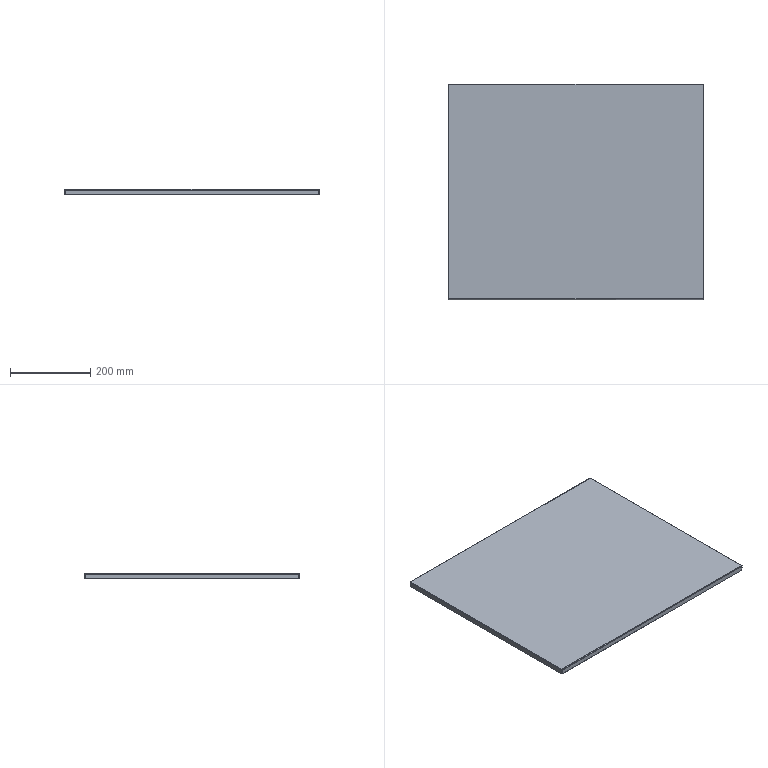Part | STEP file | Part 3^Frame unit | 1 solid | 38 faces | box 638 x 538 x 13.5 mm | volume 554979 mm3 | plane 22 | spline 8 | cylinder 8 | commonest cylinder face diameters 1 x4 4 x4
STEP:
#1=CARTESIAN_POINT('',(-317.,83.,-1.5));
#2=VERTEX_POINT('',#1);
#3=CARTESIAN_POINT('',(317.,83.,-1.5));
#4=VERTEX_POINT('',#3);
#5=CARTESIAN_POINT('',(-317.,83.,-1.5));
#6=DIRECTION('',(1.,0.,0.));
#7=VECTOR('',#6,1000.);
#8=LINE('',#5,#7);
#9=EDGE_CURVE('',#2,#4,#8,.T.);
#10=ORIENTED_EDGE('',*,*,#9,.F.);
#11=CARTESIAN_POINT('',(-317.,617.,-1.5));
#12=VERTEX_POINT('',#11);
#13=CARTESIAN_POINT('',(-317.,617.,-1.5));
#14=DIRECTION('',(0.,-1.,0.));
#15=VECTOR('',#14,1000.);
#16=LINE('',#13,#15);
#17=EDGE_CURVE('',#12,#2,#16,.T.);
#18=ORIENTED_EDGE('',*,*,#17,.F.);
#19=CARTESIAN_POINT('',(317.,617.,-1.5));
#20=VERTEX_POINT('',#19);
#21=CARTESIAN_POINT('',(317.,617.,-1.5));
#22=DIRECTION('',(-1.,0.,0.));
#23=VECTOR('',#22,1000.);
#24=LINE('',#21,#23);
#25=EDGE_CURVE('',#20,#12,#24,.T.);
#26=ORIENTED_EDGE('',*,*,#25,.F.);
#27=CARTESIAN_POINT('',(317.,83.,-1.5));
#28=DIRECTION('',(0.,1.,0.));
#29=VECTOR('',#28,1000.);
#30=LINE('',#27,#29);
#31=EDGE_CURVE('',#4,#20,#30,.T.);
#32=ORIENTED_EDGE('',*,*,#31,.F.);
#33=EDGE_LOOP('',(#10,#18,#26,#32));
#34=FACE_OUTER_BOUND('',#33,.T.);
#35=CARTESIAN_POINT('',(0.,0.,-1.5));
#36=DIRECTION('',(0.,0.,1.));
#37=DIRECTION('',(1.,0.,0.));
#38=AXIS2_PLACEMENT_3D('',#35,#36,#37);
#39=PLANE('',#38);
#40=ADVANCED_FACE('',(#34),#39,.F.);
#41=CARTESIAN_POINT('',(-317.,617.,0.));
#42=VERTEX_POINT('',#41);
#43=CARTESIAN_POINT('',(-317.,83.,0.));
#44=VERTEX_POINT('',#43);
#45=CARTESIAN_POINT('',(-317.,617.,0.));
#46=DIRECTION('',(0.,-1.,0.));
#47=VECTOR('',#46,1000.);
#48=LINE('',#45,#47);
#49=EDGE_CURVE('',#42,#44,#48,.T.);
#50=ORIENTED_EDGE('',*,*,#49,.T.);
#51=CARTESIAN_POINT('',(317.,83.,0.));
#52=VERTEX_POINT('',#51);
#53=CARTESIAN_POINT('',(-317.,83.,0.));
#54=DIRECTION('',(1.,0.,0.));
#55=VECTOR('',#54,1000.);
#56=LINE('',#53,#55);
#57=EDGE_CURVE('',#44,#52,#56,.T.);
#58=ORIENTED_EDGE('',*,*,#57,.T.);
#59=CARTESIAN_POINT('',(317.,617.,0.));
#60=VERTEX_POINT('',#59);
#61=CARTESIAN_POINT('',(317.,83.,0.));
#62=DIRECTION('',(0.,1.,0.));
#63=VECTOR('',#62,1000.);
#64=LINE('',#61,#63);
#65=EDGE_CURVE('',#52,#60,#64,.T.);
#66=ORIENTED_EDGE('',*,*,#65,.T.);
#67=CARTESIAN_POINT('',(317.,617.,0.));
#68=DIRECTION('',(-1.,0.,0.));
#69=VECTOR('',#68,1000.);
#70=LINE('',#67,#69);
#71=EDGE_CURVE('',#60,#42,#70,.T.);
#72=ORIENTED_EDGE('',*,*,#71,.T.);
#73=EDGE_LOOP('',(#50,#58,#66,#72));
#74=FACE_OUTER_BOUND('',#73,.T.);
#75=CARTESIAN_POINT('',(0.,0.,0.));
#76=DIRECTION('',(0.,0.,1.));
#77=DIRECTION('',(1.,0.,0.));
#78=AXIS2_PLACEMENT_3D('',#75,#76,#77);
#79=PLANE('',#78);
#80=ADVANCED_FACE('',(#74),#79,.T.);
#81=CARTESIAN_POINT('',(-316.793,619.,-2.));
#82=VERTEX_POINT('',#81);
#83=CARTESIAN_POINT('',(-316.793,617.5,-2.));
#84=VERTEX_POINT('',#83);
#85=CARTESIAN_POINT('',(-316.793,617.5,-2.));
#86=DIRECTION('',(0.,-1.,0.));
#87=VECTOR('',#86,1000.);
#88=LINE('',#85,#87);
#89=EDGE_CURVE('',#82,#84,#88,.T.);
#90=ORIENTED_EDGE('',*,*,#89,.T.);
#91=CARTESIAN_POINT('',(-317.,617.,-1.5));
#92=CARTESIAN_POINT('',(-316.965,617.131,-1.5));
#93=CARTESIAN_POINT('',(-316.931,617.261,-1.554));
#94=CARTESIAN_POINT('',(-316.862,617.446,-1.739));
#95=CARTESIAN_POINT('',(-316.827,617.5,-1.869));
#96=CARTESIAN_POINT('',(-316.793,617.5,-2.));
#97=B_SPLINE_CURVE_WITH_KNOTS('',3,(#91,#92,#93,#94,#95,#96),.UNSPECIFIED.,.F.,.F.,(4,2,4),(0.,0.5,1.),.UNSPECIFIED.);
#98=EDGE_CURVE('',#12,#84,#97,.T.);
#99=ORIENTED_EDGE('',*,*,#98,.F.);
#100=CARTESIAN_POINT('',(-317.,617.,-1.5));
#101=DIRECTION('',(0.,0.,1.));
#102=VECTOR('',#101,1000.);
#103=LINE('',#100,#102);
#104=EDGE_CURVE('',#12,#42,#103,.T.);
#105=ORIENTED_EDGE('',*,*,#104,.T.);
#106=CARTESIAN_POINT('',(-317.,617.,0.));
#107=CARTESIAN_POINT('',(-316.983,617.262,0.));
#108=CARTESIAN_POINT('',(-316.965,617.523,-0.05205));
#109=CARTESIAN_POINT('',(-316.931,618.007,-0.2524));
#110=CARTESIAN_POINT('',(-316.914,618.229,-0.4007));
#111=CARTESIAN_POINT('',(-316.879,618.599,-0.7709));
#112=CARTESIAN_POINT('',(-316.862,618.748,-0.9928));
#113=CARTESIAN_POINT('',(-316.827,618.948,-1.477));
#114=CARTESIAN_POINT('',(-316.81,619.,-1.738));
#115=CARTESIAN_POINT('',(-316.793,619.,-2.));
#116=B_SPLINE_CURVE_WITH_KNOTS('',3,(#106,#107,#108,#109,#110,#111,#112,#113,#114,#115),.UNSPECIFIED.,.F.,.F.,(4,2,2,2,4),(0.,0.25,0.5,0.75,1.),.UNSPECIFIED.);
#117=EDGE_CURVE('',#42,#82,#116,.T.);
#118=ORIENTED_EDGE('',*,*,#117,.T.);
#119=EDGE_LOOP('',(#90,#99,#105,#118));
#120=FACE_OUTER_BOUND('',#119,.T.);
#121=CARTESIAN_POINT('',(-317.,617.,0.015));
#122=CARTESIAN_POINT('',(-316.983,617.264,0.015));
#123=CARTESIAN_POINT('',(-316.965,617.527,-0.03745));
#124=CARTESIAN_POINT('',(-316.931,618.015,-0.2393));
#125=CARTESIAN_POINT('',(-316.914,618.238,-0.3887));
#126=CARTESIAN_POINT('',(-316.879,618.611,-0.7617));
#127=CARTESIAN_POINT('',(-316.862,618.761,-0.9852));
#128=CARTESIAN_POINT('',(-316.827,618.963,-1.473));
#129=CARTESIAN_POINT('',(-316.81,619.015,-1.736));
#130=CARTESIAN_POINT('',(-316.793,619.015,-2.));
#131=CARTESIAN_POINT('',(-317.,617.,0.));
#132=CARTESIAN_POINT('',(-316.983,617.262,0.));
#133=CARTESIAN_POINT('',(-316.965,617.523,-0.05205));
#134=CARTESIAN_POINT('',(-316.931,618.007,-0.2524));
#135=CARTESIAN_POINT('',(-316.914,618.229,-0.4007));
#136=CARTESIAN_POINT('',(-316.879,618.599,-0.7709));
#137=CARTESIAN_POINT('',(-316.862,618.748,-0.9928));
#138=CARTESIAN_POINT('',(-316.827,618.948,-1.477));
#139=CARTESIAN_POINT('',(-316.81,619.,-1.738));
#140=CARTESIAN_POINT('',(-316.793,619.,-2.));
#141=CARTESIAN_POINT('',(-317.,617.,-1.5));
#142=CARTESIAN_POINT('',(-316.983,617.065,-1.5));
#143=CARTESIAN_POINT('',(-316.965,617.131,-1.513));
#144=CARTESIAN_POINT('',(-316.931,617.252,-1.563));
#145=CARTESIAN_POINT('',(-316.914,617.307,-1.6));
#146=CARTESIAN_POINT('',(-316.879,617.4,-1.693));
#147=CARTESIAN_POINT('',(-316.862,617.437,-1.748));
#148=CARTESIAN_POINT('',(-316.827,617.487,-1.869));
#149=CARTESIAN_POINT('',(-316.81,617.5,-1.935));
#150=CARTESIAN_POINT('',(-316.793,617.5,-2.));
#151=CARTESIAN_POINT('',(-317.,617.,-1.515));
#152=CARTESIAN_POINT('',(-316.983,617.063,-1.515));
#153=CARTESIAN_POINT('',(-316.965,617.127,-1.528));
#154=CARTESIAN_POINT('',(-316.931,617.244,-1.576));
#155=CARTESIAN_POINT('',(-316.914,617.298,-1.612));
#156=CARTESIAN_POINT('',(-316.879,617.388,-1.702));
#157=CARTESIAN_POINT('',(-316.862,617.424,-1.756));
#158=CARTESIAN_POINT('',(-316.827,617.472,-1.873));
#159=CARTESIAN_POINT('',(-316.81,617.485,-1.937));
#160=CARTESIAN_POINT('',(-316.793,617.485,-2.));
#161=B_SPLINE_SURFACE_WITH_KNOTS('',1,3,((#121,#122,#123,#124,#125,#126,#127,#128,#129,#130),(#131,#132,#133,#134,#135,#136,#137,#138,#139,#140),(#141,#142,#143,#144,#145,#146,#147,#148,#149,#150),(#151,#152,#153,#154,#155,#156,#157,#158,#159,#160)),.UNSPECIFIED.,.F.,.F.,.F.,(2,1,1,2),(4,2,2,2,4),(-0.01,0.,1.,1.01),(0.,0.25,0.5,0.75,1.),.UNSPECIFIED.);
#162=ADVANCED_FACE('',(#120),#161,.F.);
#163=CARTESIAN_POINT('',(316.793,617.5,-2.));
#164=VERTEX_POINT('',#163);
#165=CARTESIAN_POINT('',(316.793,617.5,-2.));
#166=CARTESIAN_POINT('',(316.827,617.5,-1.869));
#167=CARTESIAN_POINT('',(316.862,617.446,-1.739));
#168=CARTESIAN_POINT('',(316.931,617.261,-1.554));
#169=CARTESIAN_POINT('',(316.965,617.131,-1.5));
#170=CARTESIAN_POINT('',(317.,617.,-1.5));
#171=B_SPLINE_CURVE_WITH_KNOTS('',3,(#165,#166,#167,#168,#169,#170),.UNSPECIFIED.,.F.,.F.,(4,2,4),(0.,0.5,1.),.UNSPECIFIED.);
#172=EDGE_CURVE('',#164,#20,#171,.T.);
#173=ORIENTED_EDGE('',*,*,#172,.F.);
#174=CARTESIAN_POINT('',(316.793,619.,-2.));
#175=VERTEX_POINT('',#174);
#176=CARTESIAN_POINT('',(316.793,617.5,-2.));
#177=DIRECTION('',(0.,-1.,0.));
#178=VECTOR('',#177,1000.);
#179=LINE('',#176,#178);
#180=EDGE_CURVE('',#175,#164,#179,.T.);
#181=ORIENTED_EDGE('',*,*,#180,.F.);
#182=CARTESIAN_POINT('',(316.793,619.,-2.));
#183=CARTESIAN_POINT('',(316.81,619.,-1.738));
#184=CARTESIAN_POINT('',(316.827,618.948,-1.477));
#185=CARTESIAN_POINT('',(316.862,618.748,-0.9928));
#186=CARTESIAN_POINT('',(316.879,618.599,-0.7709));
#187=CARTESIAN_POINT('',(316.914,618.229,-0.4007));
#188=CARTESIAN_POINT('',(316.931,618.007,-0.2524));
#189=CARTESIAN_POINT('',(316.965,617.523,-0.05205));
#190=CARTESIAN_POINT('',(316.983,617.262,0.));
#191=CARTESIAN_POINT('',(317.,617.,0.));
#192=B_SPLINE_CURVE_WITH_KNOTS('',3,(#182,#183,#184,#185,#186,#187,#188,#189,#190,#191),.UNSPECIFIED.,.F.,.F.,(4,2,2,2,4),(0.,0.25,0.5,0.75,1.),.UNSPECIFIED.);
#193=EDGE_CURVE('',#175,#60,#192,.T.);
#194=ORIENTED_EDGE('',*,*,#193,.T.);
#195=CARTESIAN_POINT('',(317.,617.,-1.5));
#196=DIRECTION('',(0.,0.,1.));
#197=VECTOR('',#196,1000.);
#198=LINE('',#195,#197);
#199=EDGE_CURVE('',#20,#60,#198,.T.);
#200=ORIENTED_EDGE('',*,*,#199,.F.);
#201=EDGE_LOOP('',(#173,#181,#194,#200));
#202=FACE_OUTER_BOUND('',#201,.T.);
#203=CARTESIAN_POINT('',(316.793,619.015,-2.));
#204=CARTESIAN_POINT('',(316.81,619.015,-1.736));
#205=CARTESIAN_POINT('',(316.827,618.963,-1.473));
#206=CARTESIAN_POINT('',(316.862,618.761,-0.9852));
#207=CARTESIAN_POINT('',(316.879,618.611,-0.7617));
#208=CARTESIAN_POINT('',(316.914,618.238,-0.3887));
#209=CARTESIAN_POINT('',(316.931,618.015,-0.2393));
#210=CARTESIAN_POINT('',(316.965,617.527,-0.03745));
#211=CARTESIAN_POINT('',(316.983,617.264,0.015));
#212=CARTESIAN_POINT('',(317.,617.,0.015));
#213=CARTESIAN_POINT('',(316.793,619.,-2.));
#214=CARTESIAN_POINT('',(316.81,619.,-1.738));
#215=CARTESIAN_POINT('',(316.827,618.948,-1.477));
#216=CARTESIAN_POINT('',(316.862,618.748,-0.9928));
#217=CARTESIAN_POINT('',(316.879,618.599,-0.7709));
#218=CARTESIAN_POINT('',(316.914,618.229,-0.4007));
#219=CARTESIAN_POINT('',(316.931,618.007,-0.2524));
#220=CARTESIAN_POINT('',(316.965,617.523,-0.05205));
#221=CARTESIAN_POINT('',(316.983,617.262,0.));
#222=CARTESIAN_POINT('',(317.,617.,0.));
#223=CARTESIAN_POINT('',(316.793,617.5,-2.));
#224=CARTESIAN_POINT('',(316.81,617.5,-1.935));
#225=CARTESIAN_POINT('',(316.827,617.487,-1.869));
#226=CARTESIAN_POINT('',(316.862,617.437,-1.748));
#227=CARTESIAN_POINT('',(316.879,617.4,-1.693));
#228=CARTESIAN_POINT('',(316.914,617.307,-1.6));
#229=CARTESIAN_POINT('',(316.931,617.252,-1.563));
#230=CARTESIAN_POINT('',(316.965,617.131,-1.513));
#231=CARTESIAN_POINT('',(316.983,617.065,-1.5));
#232=CARTESIAN_POINT('',(317.,617.,-1.5));
#233=CARTESIAN_POINT('',(316.793,617.485,-2.));
#234=CARTESIAN_POINT('',(316.81,617.485,-1.937));
#235=CARTESIAN_POINT('',(316.827,617.472,-1.873));
#236=CARTESIAN_POINT('',(316.862,617.424,-1.756));
#237=CARTESIAN_POINT('',(316.879,617.388,-1.702));
#238=CARTESIAN_POINT('',(316.914,617.298,-1.612));
#239=CARTESIAN_POINT('',(316.931,617.244,-1.576));
#240=CARTESIAN_POINT('',(316.965,617.127,-1.528));
#241=CARTESIAN_POINT('',(316.983,617.063,-1.515));
#242=CARTESIAN_POINT('',(317.,617.,-1.515));
#243=B_SPLINE_SURFACE_WITH_KNOTS('',1,3,((#203,#204,#205,#206,#207,#208,#209,#210,#211,#212),(#213,#214,#215,#216,#217,#218,#219,#220,#221,#222),(#223,#224,#225,#226,#227,#228,#229,#230,#231,#232),(#233,#234,#235,#236,#237,#238,#239,#240,#241,#242)),.UNSPECIFIED.,.F.,.F.,.F.,(2,1,1,2),(4,2,2,2,4),(-0.01,0.,1.,1.01),(0.,0.25,0.5,0.75,1.),.UNSPECIFIED.);
#244=ADVANCED_FACE('',(#202),#243,.F.);
#245=ORIENTED_EDGE('',*,*,#71,.F.);
#246=ORIENTED_EDGE('',*,*,#193,.F.);
#247=CARTESIAN_POINT('',(-319.,619.,-2.));
#248=DIRECTION('',(-1.,0.,0.));
#249=VECTOR('',#248,1000.);
#250=LINE('',#247,#249);
#251=EDGE_CURVE('',#175,#82,#250,.T.);
#252=ORIENTED_EDGE('',*,*,#251,.T.);
#253=ORIENTED_EDGE('',*,*,#117,.F.);
#254=EDGE_LOOP('',(#245,#246,#252,#253));
#255=FACE_OUTER_BOUND('',#254,.T.);
#256=CARTESIAN_POINT('',(317.,617.,-2.));
#257=DIRECTION('',(1.,0.,0.));
#258=DIRECTION('',(0.,1.,0.));
#259=AXIS2_PLACEMENT_3D('',#256,#257,#258);
#260=CYLINDRICAL_SURFACE('',#259,2.);
#261=ADVANCED_FACE('',(#255),#260,.T.);
#262=ORIENTED_EDGE('',*,*,#25,.T.);
#263=ORIENTED_EDGE('',*,*,#98,.T.);
#264=CARTESIAN_POINT('',(-319.,617.5,-2.));
#265=DIRECTION('',(1.,0.,0.));
#266=VECTOR('',#265,1000.);
#267=LINE('',#264,#266);
#268=EDGE_CURVE('',#84,#164,#267,.T.);
#269=ORIENTED_EDGE('',*,*,#268,.T.);
#270=ORIENTED_EDGE('',*,*,#172,.T.);
#271=EDGE_LOOP('',(#262,#263,#269,#270));
#272=FACE_OUTER_BOUND('',#271,.T.);
#273=CARTESIAN_POINT('',(317.,617.,-2.));
#274=DIRECTION('',(1.,0.,0.));
#275=DIRECTION('',(0.,1.,0.));
#276=AXIS2_PLACEMENT_3D('',#273,#274,#275);
#277=CYLINDRICAL_SURFACE('',#276,0.5);
#278=ADVANCED_FACE('',(#272),#277,.F.);
#279=CARTESIAN_POINT('',(-316.793,619.,-13.5));
#280=VERTEX_POINT('',#279);
#281=CARTESIAN_POINT('',(-316.793,619.,-1.5));
#282=DIRECTION('',(0.,0.,-1.));
#283=VECTOR('',#282,1000.);
#284=LINE('',#281,#283);
#285=EDGE_CURVE('',#82,#280,#284,.T.);
#286=ORIENTED_EDGE('',*,*,#285,.T.);
#287=CARTESIAN_POINT('',(-316.793,617.5,-13.5));
#288=VERTEX_POINT('',#287);
#289=CARTESIAN_POINT('',(-316.793,617.5,-13.5));
#290=DIRECTION('',(0.,-1.,0.));
#291=VECTOR('',#290,1000.);
#292=LINE('',#289,#291);
#293=EDGE_CURVE('',#280,#288,#292,.T.);
#294=ORIENTED_EDGE('',*,*,#293,.T.);
#295=CARTESIAN_POINT('',(-316.793,617.5,0.));
#296=DIRECTION('',(0.,0.,-1.));
#297=VECTOR('',#296,1000.);
#298=LINE('',#295,#297);
#299=EDGE_CURVE('',#84,#288,#298,.T.);
#300=ORIENTED_EDGE('',*,*,#299,.F.);
#301=ORIENTED_EDGE('',*,*,#89,.F.);
#302=EDGE_LOOP('',(#286,#294,#300,#301));
#303=FACE_OUTER_BOUND('',#302,.T.);
#304=CARTESIAN_POINT('',(-316.793,617.5,-1.5));
#305=DIRECTION('',(-1.,0.,0.));
#306=DIRECTION('',(0.,0.,1.));
#307=AXIS2_PLACEMENT_3D('',#304,#305,#306);
#308=PLANE('',#307);
#309=ADVANCED_FACE('',(#303),#308,.T.);
#310=ORIENTED_EDGE('',*,*,#285,.F.);
#311=ORIENTED_EDGE('',*,*,#251,.F.);
#312=CARTESIAN_POINT('',(316.793,619.,-13.5));
#313=VERTEX_POINT('',#312);
#314=CARTESIAN_POINT('',(316.793,619.,0.));
#315=DIRECTION('',(0.,0.,-1.));
#316=VECTOR('',#315,1000.);
#317=LINE('',#314,#316);
#318=EDGE_CURVE('',#175,#313,#317,.T.);
#319=ORIENTED_EDGE('',*,*,#318,.T.);
#320=CARTESIAN_POINT('',(0.,619.,-13.5));
#321=DIRECTION('',(-1.,0.,0.));
#322=VECTOR('',#321,1000.);
#323=LINE('',#320,#322);
#324=EDGE_CURVE('',#313,#280,#323,.T.);
#325=ORIENTED_EDGE('',*,*,#324,.T.);
#326=EDGE_LOOP('',(#310,#311,#319,#325));
#327=FACE_OUTER_BOUND('',#326,.T.);
#328=CARTESIAN_POINT('',(0.,619.,0.));
#329=DIRECTION('',(0.,-1.,0.));
#330=DIRECTION('',(0.,0.,-1.));
#331=AXIS2_PLACEMENT_3D('',#328,#329,#330);
#332=PLANE('',#331);
#333=ADVANCED_FACE('',(#327),#332,.F.);
#334=ORIENTED_EDGE('',*,*,#268,.F.);
#335=ORIENTED_EDGE('',*,*,#299,.T.);
#336=CARTESIAN_POINT('',(316.793,617.5,-13.5));
#337=VERTEX_POINT('',#336);
#338=CARTESIAN_POINT('',(-319.,617.5,-13.5));
#339=DIRECTION('',(-1.,0.,0.));
#340=VECTOR('',#339,1000.);
#341=LINE('',#338,#340);
#342=EDGE_CURVE('',#337,#288,#341,.T.);
#343=ORIENTED_EDGE('',*,*,#342,.F.);
#344=CARTESIAN_POINT('',(316.793,617.5,-1.5));
#345=DIRECTION('',(0.,0.,-1.));
#346=VECTOR('',#345,1000.);
#347=LINE('',#344,#346);
#348=EDGE_CURVE('',#164,#337,#347,.T.);
#349=ORIENTED_EDGE('',*,*,#348,.F.);
#350=EDGE_LOOP('',(#334,#335,#343,#349));
#351=FACE_OUTER_BOUND('',#350,.T.);
#352=CARTESIAN_POINT('',(0.,617.5,0.));
#353=DIRECTION('',(0.,-1.,0.));
#354=DIRECTION('',(0.,0.,-1.));
#355=AXIS2_PLACEMENT_3D('',#352,#353,#354);
#356=PLANE('',#355);
#357=ADVANCED_FACE('',(#351),#356,.T.);
#358=ORIENTED_EDGE('',*,*,#293,.F.);
#359=ORIENTED_EDGE('',*,*,#324,.F.);
#360=CARTESIAN_POINT('',(316.793,619.,-13.5));
#361=DIRECTION('',(0.,-1.,0.));
#362=VECTOR('',#361,1000.);
#363=LINE('',#360,#362);
#364=EDGE_CURVE('',#313,#337,#363,.T.);
#365=ORIENTED_EDGE('',*,*,#364,.T.);
#366=ORIENTED_EDGE('',*,*,#342,.T.);
#367=EDGE_LOOP('',(#358,#359,#365,#366));
#368=FACE_OUTER_BOUND('',#367,.T.);
#369=CARTESIAN_POINT('',(-319.,619.,-13.5));
#370=DIRECTION('',(0.,0.,1.));
#371=DIRECTION('',(0.,-1.,0.));
#372=AXIS2_PLACEMENT_3D('',#369,#370,#371);
#373=PLANE('',#372);
#374=ADVANCED_FACE('',(#368),#373,.F.);
#375=ORIENTED_EDGE('',*,*,#364,.F.);
#376=ORIENTED_EDGE('',*,*,#318,.F.);
#377=ORIENTED_EDGE('',*,*,#180,.T.);
#378=ORIENTED_EDGE('',*,*,#348,.T.);
#379=EDGE_LOOP('',(#375,#376,#377,#378));
#380=FACE_OUTER_BOUND('',#379,.T.);
#381=CARTESIAN_POINT('',(316.793,617.5,-1.5));
#382=DIRECTION('',(-1.,0.,0.));
#383=DIRECTION('',(0.,0.,1.));
#384=AXIS2_PLACEMENT_3D('',#381,#382,#383);
#385=PLANE('',#384);
#386=ADVANCED_FACE('',(#380),#385,.F.);
#387=CARTESIAN_POINT('',(-319.,83.207,-2.));
#388=VERTEX_POINT('',#387);
#389=CARTESIAN_POINT('',(-317.5,83.207,-2.));
#390=VERTEX_POINT('',#389);
#391=CARTESIAN_POINT('',(-317.5,83.207,-2.));
#392=DIRECTION('',(1.,0.,0.));
#393=VECTOR('',#392,1000.);
#394=LINE('',#391,#393);
#395=EDGE_CURVE('',#388,#390,#394,.T.);
#396=ORIENTED_EDGE('',*,*,#395,.T.);
#397=CARTESIAN_POINT('',(-317.,83.,-1.5));
#398=CARTESIAN_POINT('',(-317.131,83.035,-1.5));
#399=CARTESIAN_POINT('',(-317.261,83.069,-1.554));
#400=CARTESIAN_POINT('',(-317.446,83.138,-1.739));
#401=CARTESIAN_POINT('',(-317.5,83.173,-1.869));
#402=CARTESIAN_POINT('',(-317.5,83.207,-2.));
#403=B_SPLINE_CURVE_WITH_KNOTS('',3,(#397,#398,#399,#400,#401,#402),.UNSPECIFIED.,.F.,.F.,(4,2,4),(0.,0.5,1.),.UNSPECIFIED.);
#404=EDGE_CURVE('',#2,#390,#403,.T.);
#405=ORIENTED_EDGE('',*,*,#404,.F.);
#406=CARTESIAN_POINT('',(-317.,83.,-1.5));
#407=DIRECTION('',(0.,0.,1.));
#408=VECTOR('',#407,1000.);
#409=LINE('',#406,#408);
#410=EDGE_CURVE('',#2,#44,#409,.T.);
#411=ORIENTED_EDGE('',*,*,#410,.T.);
#412=CARTESIAN_POINT('',(-317.,83.,0.));
#413=CARTESIAN_POINT('',(-317.262,83.017,0.));
#414=CARTESIAN_POINT('',(-317.523,83.035,-0.05205));
#415=CARTESIAN_POINT('',(-318.007,83.069,-0.2524));
#416=CARTESIAN_POINT('',(-318.229,83.086,-0.4007));
#417=CARTESIAN_POINT('',(-318.599,83.121,-0.7709));
#418=CARTESIAN_POINT('',(-318.748,83.138,-0.9928));
#419=CARTESIAN_POINT('',(-318.948,83.173,-1.477));
#420=CARTESIAN_POINT('',(-319.,83.19,-1.738));
#421=CARTESIAN_POINT('',(-319.,83.207,-2.));
#422=B_SPLINE_CURVE_WITH_KNOTS('',3,(#412,#413,#414,#415,#416,#417,#418,#419,#420,#421),.UNSPECIFIED.,.F.,.F.,(4,2,2,2,4),(0.,0.25,0.5,0.75,1.),.UNSPECIFIED.);
#423=EDGE_CURVE('',#44,#388,#422,.T.);
#424=ORIENTED_EDGE('',*,*,#423,.T.);
#425=EDGE_LOOP('',(#396,#405,#411,#424));
#426=FACE_OUTER_BOUND('',#425,.T.);
#427=CARTESIAN_POINT('',(-317.,83.,0.015));
#428=CARTESIAN_POINT('',(-317.264,83.017,0.015));
#429=CARTESIAN_POINT('',(-317.527,83.035,-0.03745));
#430=CARTESIAN_POINT('',(-318.015,83.069,-0.2393));
#431=CARTESIAN_POINT('',(-318.238,83.086,-0.3887));
#432=CARTESIAN_POINT('',(-318.611,83.121,-0.7617));
#433=CARTESIAN_POINT('',(-318.761,83.138,-0.9852));
#434=CARTESIAN_POINT('',(-318.963,83.173,-1.473));
#435=CARTESIAN_POINT('',(-319.015,83.19,-1.736));
#436=CARTESIAN_POINT('',(-319.015,83.207,-2.));
#437=CARTESIAN_POINT('',(-317.,83.,0.));
#438=CARTESIAN_POINT('',(-317.262,83.017,0.));
#439=CARTESIAN_POINT('',(-317.523,83.035,-0.05205));
#440=CARTESIAN_POINT('',(-318.007,83.069,-0.2524));
#441=CARTESIAN_POINT('',(-318.229,83.086,-0.4007));
#442=CARTESIAN_POINT('',(-318.599,83.121,-0.7709));
#443=CARTESIAN_POINT('',(-318.748,83.138,-0.9928));
#444=CARTESIAN_POINT('',(-318.948,83.173,-1.477));
#445=CARTESIAN_POINT('',(-319.,83.19,-1.738));
#446=CARTESIAN_POINT('',(-319.,83.207,-2.));
#447=CARTESIAN_POINT('',(-317.,83.,-1.5));
#448=CARTESIAN_POINT('',(-317.065,83.017,-1.5));
#449=CARTESIAN_POINT('',(-317.131,83.035,-1.513));
#450=CARTESIAN_POINT('',(-317.252,83.069,-1.563));
#451=CARTESIAN_POINT('',(-317.307,83.086,-1.6));
#452=CARTESIAN_POINT('',(-317.4,83.121,-1.693));
#453=CARTESIAN_POINT('',(-317.437,83.138,-1.748));
#454=CARTESIAN_POINT('',(-317.487,83.173,-1.869));
#455=CARTESIAN_POINT('',(-317.5,83.19,-1.935));
#456=CARTESIAN_POINT('',(-317.5,83.207,-2.));
#457=CARTESIAN_POINT('',(-317.,83.,-1.515));
#458=CARTESIAN_POINT('',(-317.063,83.017,-1.515));
#459=CARTESIAN_POINT('',(-317.127,83.035,-1.528));
#460=CARTESIAN_POINT('',(-317.244,83.069,-1.576));
#461=CARTESIAN_POINT('',(-317.298,83.086,-1.612));
#462=CARTESIAN_POINT('',(-317.388,83.121,-1.702));
#463=CARTESIAN_POINT('',(-317.424,83.138,-1.756));
#464=CARTESIAN_POINT('',(-317.472,83.173,-1.873));
#465=CARTESIAN_POINT('',(-317.485,83.19,-1.937));
#466=CARTESIAN_POINT('',(-317.485,83.207,-2.));
#467=B_SPLINE_SURFACE_WITH_KNOTS('',1,3,((#427,#428,#429,#430,#431,#432,#433,#434,#435,#436),(#437,#438,#439,#440,#441,#442,#443,#444,#445,#446),(#447,#448,#449,#450,#451,#452,#453,#454,#455,#456),(#457,#458,#459,#460,#461,#462,#463,#464,#465,#466)),.UNSPECIFIED.,.F.,.F.,.F.,(2,1,1,2),(4,2,2,2,4),(-0.01,0.,1.,1.01),(0.,0.25,0.5,0.75,1.),.UNSPECIFIED.);
#468=ADVANCED_FACE('',(#426),#467,.F.);
#469=CARTESIAN_POINT('',(-317.5,616.793,-2.));
#470=VERTEX_POINT('',#469);
#471=CARTESIAN_POINT('',(-317.5,616.793,-2.));
#472=CARTESIAN_POINT('',(-317.5,616.827,-1.869));
#473=CARTESIAN_POINT('',(-317.446,616.862,-1.739));
#474=CARTESIAN_POINT('',(-317.261,616.931,-1.554));
#475=CARTESIAN_POINT('',(-317.131,616.965,-1.5));
#476=CARTESIAN_POINT('',(-317.,617.,-1.5));
#477=B_SPLINE_CURVE_WITH_KNOTS('',3,(#471,#472,#473,#474,#475,#476),.UNSPECIFIED.,.F.,.F.,(4,2,4),(0.,0.5,1.),.UNSPECIFIED.);
#478=EDGE_CURVE('',#470,#12,#477,.T.);
#479=ORIENTED_EDGE('',*,*,#478,.F.);
#480=CARTESIAN_POINT('',(-319.,616.793,-2.));
#481=VERTEX_POINT('',#480);
#482=CARTESIAN_POINT('',(-317.5,616.793,-2.));
#483=DIRECTION('',(1.,0.,0.));
#484=VECTOR('',#483,1000.);
#485=LINE('',#482,#484);
#486=EDGE_CURVE('',#481,#470,#485,.T.);
#487=ORIENTED_EDGE('',*,*,#486,.F.);
#488=CARTESIAN_POINT('',(-319.,616.793,-2.));
#489=CARTESIAN_POINT('',(-319.,616.81,-1.738));
#490=CARTESIAN_POINT('',(-318.948,616.827,-1.477));
#491=CARTESIAN_POINT('',(-318.748,616.862,-0.9928));
#492=CARTESIAN_POINT('',(-318.599,616.879,-0.7709));
#493=CARTESIAN_POINT('',(-318.229,616.914,-0.4007));
#494=CARTESIAN_POINT('',(-318.007,616.931,-0.2524));
#495=CARTESIAN_POINT('',(-317.523,616.965,-0.05205));
#496=CARTESIAN_POINT('',(-317.262,616.983,0.));
#497=CARTESIAN_POINT('',(-317.,617.,0.));
#498=B_SPLINE_CURVE_WITH_KNOTS('',3,(#488,#489,#490,#491,#492,#493,#494,#495,#496,#497),.UNSPECIFIED.,.F.,.F.,(4,2,2,2,4),(0.,0.25,0.5,0.75,1.),.UNSPECIFIED.);
#499=EDGE_CURVE('',#481,#42,#498,.T.);
#500=ORIENTED_EDGE('',*,*,#499,.T.);
#501=ORIENTED_EDGE('',*,*,#104,.F.);
#502=EDGE_LOOP('',(#479,#487,#500,#501));
#503=FACE_OUTER_BOUND('',#502,.T.);
#504=CARTESIAN_POINT('',(-319.015,616.793,-2.));
#505=CARTESIAN_POINT('',(-319.015,616.81,-1.736));
#506=CARTESIAN_POINT('',(-318.963,616.827,-1.473));
#507=CARTESIAN_POINT('',(-318.761,616.862,-0.9852));
#508=CARTESIAN_POINT('',(-318.611,616.879,-0.7617));
#509=CARTESIAN_POINT('',(-318.238,616.914,-0.3887));
#510=CARTESIAN_POINT('',(-318.015,616.931,-0.2393));
#511=CARTESIAN_POINT('',(-317.527,616.965,-0.03745));
#512=CARTESIAN_POINT('',(-317.264,616.983,0.015));
#513=CARTESIAN_POINT('',(-317.,617.,0.015));
#514=CARTESIAN_POINT('',(-319.,616.793,-2.));
#515=CARTESIAN_POINT('',(-319.,616.81,-1.738));
#516=CARTESIAN_POINT('',(-318.948,616.827,-1.477));
#517=CARTESIAN_POINT('',(-318.748,616.862,-0.9928));
#518=CARTESIAN_POINT('',(-318.599,616.879,-0.7709));
#519=CARTESIAN_POINT('',(-318.229,616.914,-0.4007));
#520=CARTESIAN_POINT('',(-318.007,616.931,-0.2524));
#521=CARTESIAN_POINT('',(-317.523,616.965,-0.05205));
#522=CARTESIAN_POINT('',(-317.262,616.983,0.));
#523=CARTESIAN_POINT('',(-317.,617.,0.));
#524=CARTESIAN_POINT('',(-317.5,616.793,-2.));
#525=CARTESIAN_POINT('',(-317.5,616.81,-1.935));
#526=CARTESIAN_POINT('',(-317.487,616.827,-1.869));
#527=CARTESIAN_POINT('',(-317.437,616.862,-1.748));
#528=CARTESIAN_POINT('',(-317.4,616.879,-1.693));
#529=CARTESIAN_POINT('',(-317.307,616.914,-1.6));
#530=CARTESIAN_POINT('',(-317.252,616.931,-1.563));
#531=CARTESIAN_POINT('',(-317.131,616.965,-1.513));
#532=CARTESIAN_POINT('',(-317.065,616.983,-1.5));
#533=CARTESIAN_POINT('',(-317.,617.,-1.5));
#534=CARTESIAN_POINT('',(-317.485,616.793,-2.));
#535=CARTESIAN_POINT('',(-317.485,616.81,-1.937));
#536=CARTESIAN_POINT('',(-317.472,616.827,-1.873));
#537=CARTESIAN_POINT('',(-317.424,616.862,-1.756));
#538=CARTESIAN_POINT('',(-317.388,616.879,-1.702));
#539=CARTESIAN_POINT('',(-317.298,616.914,-1.612));
#540=CARTESIAN_POINT('',(-317.244,616.931,-1.576));
#541=CARTESIAN_POINT('',(-317.127,616.965,-1.528));
#542=CARTESIAN_POINT('',(-317.063,616.983,-1.515));
#543=CARTESIAN_POINT('',(-317.,617.,-1.515));
#544=B_SPLINE_SURFACE_WITH_KNOTS('',1,3,((#504,#505,#506,#507,#508,#509,#510,#511,#512,#513),(#514,#515,#516,#517,#518,#519,#520,#521,#522,#523),(#524,#525,#526,#527,#528,#529,#530,#531,#532,#533),(#534,#535,#536,#537,#538,#539,#540,#541,#542,#543)),.UNSPECIFIED.,.F.,.F.,.F.,(2,1,1,2),(4,2,2,2,4),(-0.01,0.,1.,1.01),(0.,0.25,0.5,0.75,1.),.UNSPECIFIED.);
#545=ADVANCED_FACE('',(#503),#544,.F.);
#546=ORIENTED_EDGE('',*,*,#49,.F.);
#547=ORIENTED_EDGE('',*,*,#499,.F.);
#548=CARTESIAN_POINT('',(-319.,81.,-2.));
#549=DIRECTION('',(0.,-1.,0.));
#550=VECTOR('',#549,1000.);
#551=LINE('',#548,#550);
#552=EDGE_CURVE('',#481,#388,#551,.T.);
#553=ORIENTED_EDGE('',*,*,#552,.T.);
#554=ORIENTED_EDGE('',*,*,#423,.F.);
#555=EDGE_LOOP('',(#546,#547,#553,#554));
#556=FACE_OUTER_BOUND('',#555,.T.);
#557=CARTESIAN_POINT('',(-317.,617.,-2.));
#558=DIRECTION('',(0.,1.,0.));
#559=DIRECTION('',(-1.,0.,0.));
#560=AXIS2_PLACEMENT_3D('',#557,#558,#559);
#561=CYLINDRICAL_SURFACE('',#560,2.);
#562=ADVANCED_FACE('',(#556),#561,.T.);
#563=ORIENTED_EDGE('',*,*,#17,.T.);
#564=ORIENTED_EDGE('',*,*,#404,.T.);
#565=CARTESIAN_POINT('',(-317.5,81.,-2.));
#566=DIRECTION('',(0.,1.,0.));
#567=VECTOR('',#566,1000.);
#568=LINE('',#565,#567);
#569=EDGE_CURVE('',#390,#470,#568,.T.);
#570=ORIENTED_EDGE('',*,*,#569,.T.);
#571=ORIENTED_EDGE('',*,*,#478,.T.);
#572=EDGE_LOOP('',(#563,#564,#570,#571));
#573=FACE_OUTER_BOUND('',#572,.T.);
#574=CARTESIAN_POINT('',(-317.,617.,-2.));
#575=DIRECTION('',(0.,1.,0.));
#576=DIRECTION('',(-1.,0.,0.));
#577=AXIS2_PLACEMENT_3D('',#574,#575,#576);
#578=CYLINDRICAL_SURFACE('',#577,0.5);
#579=ADVANCED_FACE('',(#573),#578,.F.);
#580=CARTESIAN_POINT('',(-319.,83.207,-13.5));
#581=VERTEX_POINT('',#580);
#582=CARTESIAN_POINT('',(-319.,83.207,-1.5));
#583=DIRECTION('',(0.,0.,-1.));
#584=VECTOR('',#583,1000.);
#585=LINE('',#582,#584);
#586=EDGE_CURVE('',#388,#581,#585,.T.);
#587=ORIENTED_EDGE('',*,*,#586,.T.);
#588=CARTESIAN_POINT('',(-317.5,83.207,-13.5));
#589=VERTEX_POINT('',#588);
#590=CARTESIAN_POINT('',(-317.5,83.207,-13.5));
#591=DIRECTION('',(1.,0.,0.));
#592=VECTOR('',#591,1000.);
#593=LINE('',#590,#592);
#594=EDGE_CURVE('',#581,#589,#593,.T.);
#595=ORIENTED_EDGE('',*,*,#594,.T.);
#596=CARTESIAN_POINT('',(-317.5,83.207,0.));
#597=DIRECTION('',(0.,0.,-1.));
#598=VECTOR('',#597,1000.);
#599=LINE('',#596,#598);
#600=EDGE_CURVE('',#390,#589,#599,.T.);
#601=ORIENTED_EDGE('',*,*,#600,.F.);
#602=ORIENTED_EDGE('',*,*,#395,.F.);
#603=EDGE_LOOP('',(#587,#595,#601,#602));
#604=FACE_OUTER_BOUND('',#603,.T.);
#605=CARTESIAN_POINT('',(-317.5,83.207,-1.5));
#606=DIRECTION('',(0.,-1.,0.));
#607=DIRECTION('',(0.,0.,-1.));
#608=AXIS2_PLACEMENT_3D('',#605,#606,#607);
#609=PLANE('',#608);
#610=ADVANCED_FACE('',(#604),#609,.T.);
#611=ORIENTED_EDGE('',*,*,#586,.F.);
#612=ORIENTED_EDGE('',*,*,#552,.F.);
#613=CARTESIAN_POINT('',(-319.,616.793,-13.5));
#614=VERTEX_POINT('',#613);
#615=CARTESIAN_POINT('',(-319.,616.793,0.));
#616=DIRECTION('',(0.,0.,-1.));
#617=VECTOR('',#616,1000.);
#618=LINE('',#615,#617);
#619=EDGE_CURVE('',#481,#614,#618,.T.);
#620=ORIENTED_EDGE('',*,*,#619,.T.);
#621=CARTESIAN_POINT('',(-319.,0.,-13.5));
#622=DIRECTION('',(0.,-1.,0.));
#623=VECTOR('',#622,1000.);
#624=LINE('',#621,#623);
#625=EDGE_CURVE('',#614,#581,#624,.T.);
#626=ORIENTED_EDGE('',*,*,#625,.T.);
#627=EDGE_LOOP('',(#611,#612,#620,#626));
#628=FACE_OUTER_BOUND('',#627,.T.);
#629=CARTESIAN_POINT('',(-319.,0.,0.));
#630=DIRECTION('',(1.,0.,0.));
#631=DIRECTION('',(0.,0.,-1.));
#632=AXIS2_PLACEMENT_3D('',#629,#630,#631);
#633=PLANE('',#632);
#634=ADVANCED_FACE('',(#628),#633,.F.);
#635=ORIENTED_EDGE('',*,*,#569,.F.);
#636=ORIENTED_EDGE('',*,*,#600,.T.);
#637=CARTESIAN_POINT('',(-317.5,616.793,-13.5));
#638=VERTEX_POINT('',#637);
#639=CARTESIAN_POINT('',(-317.5,81.,-13.5));
#640=DIRECTION('',(0.,-1.,0.));
#641=VECTOR('',#640,1000.);
#642=LINE('',#639,#641);
#643=EDGE_CURVE('',#638,#589,#642,.T.);
#644=ORIENTED_EDGE('',*,*,#643,.F.);
#645=CARTESIAN_POINT('',(-317.5,616.793,-1.5));
#646=DIRECTION('',(0.,0.,-1.));
#647=VECTOR('',#646,1000.);
#648=LINE('',#645,#647);
#649=EDGE_CURVE('',#470,#638,#648,.T.);
#650=ORIENTED_EDGE('',*,*,#649,.F.);
#651=EDGE_LOOP('',(#635,#636,#644,#650));
#652=FACE_OUTER_BOUND('',#651,.T.);
#653=CARTESIAN_POINT('',(-317.5,0.,0.));
#654=DIRECTION('',(1.,0.,0.));
#655=DIRECTION('',(0.,0.,-1.));
#656=AXIS2_PLACEMENT_3D('',#653,#654,#655);
#657=PLANE('',#656);
#658=ADVANCED_FACE('',(#652),#657,.T.);
#659=ORIENTED_EDGE('',*,*,#594,.F.);
#660=ORIENTED_EDGE('',*,*,#625,.F.);
#661=CARTESIAN_POINT('',(-319.,616.793,-13.5));
#662=DIRECTION('',(1.,0.,0.));
#663=VECTOR('',#662,1000.);
#664=LINE('',#661,#663);
#665=EDGE_CURVE('',#614,#638,#664,.T.);
#666=ORIENTED_EDGE('',*,*,#665,.T.);
#667=ORIENTED_EDGE('',*,*,#643,.T.);
#668=EDGE_LOOP('',(#659,#660,#666,#667));
#669=FACE_OUTER_BOUND('',#668,.T.);
#670=CARTESIAN_POINT('',(-319.,81.,-13.5));
#671=DIRECTION('',(0.,0.,1.));
#672=DIRECTION('',(1.,0.,0.));
#673=AXIS2_PLACEMENT_3D('',#670,#671,#672);
#674=PLANE('',#673);
#675=ADVANCED_FACE('',(#669),#674,.F.);
#676=ORIENTED_EDGE('',*,*,#665,.F.);
#677=ORIENTED_EDGE('',*,*,#619,.F.);
#678=ORIENTED_EDGE('',*,*,#486,.T.);
#679=ORIENTED_EDGE('',*,*,#649,.T.);
#680=EDGE_LOOP('',(#676,#677,#678,#679));
#681=FACE_OUTER_BOUND('',#680,.T.);
#682=CARTESIAN_POINT('',(-317.5,616.793,-1.5));
#683=DIRECTION('',(0.,-1.,0.));
#684=DIRECTION('',(0.,0.,-1.));
#685=AXIS2_PLACEMENT_3D('',#682,#683,#684);
#686=PLANE('',#685);
#687=ADVANCED_FACE('',(#681),#686,.F.);
#688=CARTESIAN_POINT('',(319.,616.793,-2.));
#689=VERTEX_POINT('',#688);
#690=CARTESIAN_POINT('',(317.5,616.793,-2.));
#691=VERTEX_POINT('',#690);
#692=CARTESIAN_POINT('',(317.5,616.793,-2.));
#693=DIRECTION('',(-1.,0.,0.));
#694=VECTOR('',#693,1000.);
#695=LINE('',#692,#694);
#696=EDGE_CURVE('',#689,#691,#695,.T.);
#697=ORIENTED_EDGE('',*,*,#696,.T.);
#698=CARTESIAN_POINT('',(317.,617.,-1.5));
#699=CARTESIAN_POINT('',(317.131,616.965,-1.5));
#700=CARTESIAN_POINT('',(317.261,616.931,-1.554));
#701=CARTESIAN_POINT('',(317.446,616.862,-1.739));
#702=CARTESIAN_POINT('',(317.5,616.827,-1.869));
#703=CARTESIAN_POINT('',(317.5,616.793,-2.));
#704=B_SPLINE_CURVE_WITH_KNOTS('',3,(#698,#699,#700,#701,#702,#703),.UNSPECIFIED.,.F.,.F.,(4,2,4),(0.,0.5,1.),.UNSPECIFIED.);
#705=EDGE_CURVE('',#20,#691,#704,.T.);
#706=ORIENTED_EDGE('',*,*,#705,.F.);
#707=ORIENTED_EDGE('',*,*,#199,.T.);
#708=CARTESIAN_POINT('',(317.,617.,0.));
#709=CARTESIAN_POINT('',(317.262,616.983,0.));
#710=CARTESIAN_POINT('',(317.523,616.965,-0.05205));
#711=CARTESIAN_POINT('',(318.007,616.931,-0.2524));
#712=CARTESIAN_POINT('',(318.229,616.914,-0.4007));
#713=CARTESIAN_POINT('',(318.599,616.879,-0.7709));
#714=CARTESIAN_POINT('',(318.748,616.862,-0.9928));
#715=CARTESIAN_POINT('',(318.948,616.827,-1.477));
#716=CARTESIAN_POINT('',(319.,616.81,-1.738));
#717=CARTESIAN_POINT('',(319.,616.793,-2.));
#718=B_SPLINE_CURVE_WITH_KNOTS('',3,(#708,#709,#710,#711,#712,#713,#714,#715,#716,#717),.UNSPECIFIED.,.F.,.F.,(4,2,2,2,4),(0.,0.25,0.5,0.75,1.),.UNSPECIFIED.);
#719=EDGE_CURVE('',#60,#689,#718,.T.);
#720=ORIENTED_EDGE('',*,*,#719,.T.);
#721=EDGE_LOOP('',(#697,#706,#707,#720));
#722=FACE_OUTER_BOUND('',#721,.T.);
#723=CARTESIAN_POINT('',(317.,617.,0.015));
#724=CARTESIAN_POINT('',(317.264,616.983,0.015));
#725=CARTESIAN_POINT('',(317.527,616.965,-0.03745));
#726=CARTESIAN_POINT('',(318.015,616.931,-0.2393));
#727=CARTESIAN_POINT('',(318.238,616.914,-0.3887));
#728=CARTESIAN_POINT('',(318.611,616.879,-0.7617));
#729=CARTESIAN_POINT('',(318.761,616.862,-0.9852));
#730=CARTESIAN_POINT('',(318.963,616.827,-1.473));
#731=CARTESIAN_POINT('',(319.015,616.81,-1.736));
#732=CARTESIAN_POINT('',(319.015,616.793,-2.));
#733=CARTESIAN_POINT('',(317.,617.,0.));
#734=CARTESIAN_POINT('',(317.262,616.983,0.));
#735=CARTESIAN_POINT('',(317.523,616.965,-0.05205));
#736=CARTESIAN_POINT('',(318.007,616.931,-0.2524));
#737=CARTESIAN_POINT('',(318.229,616.914,-0.4007));
#738=CARTESIAN_POINT('',(318.599,616.879,-0.7709));
#739=CARTESIAN_POINT('',(318.748,616.862,-0.9928));
#740=CARTESIAN_POINT('',(318.948,616.827,-1.477));
#741=CARTESIAN_POINT('',(319.,616.81,-1.738));
#742=CARTESIAN_POINT('',(319.,616.793,-2.));
#743=CARTESIAN_POINT('',(317.,617.,-1.5));
#744=CARTESIAN_POINT('',(317.065,616.983,-1.5));
#745=CARTESIAN_POINT('',(317.131,616.965,-1.513));
#746=CARTESIAN_POINT('',(317.252,616.931,-1.563));
#747=CARTESIAN_POINT('',(317.307,616.914,-1.6));
#748=CARTESIAN_POINT('',(317.4,616.879,-1.693));
#749=CARTESIAN_POINT('',(317.437,616.862,-1.748));
#750=CARTESIAN_POINT('',(317.487,616.827,-1.869));
#751=CARTESIAN_POINT('',(317.5,616.81,-1.935));
#752=CARTESIAN_POINT('',(317.5,616.793,-2.));
#753=CARTESIAN_POINT('',(317.,617.,-1.515));
#754=CARTESIAN_POINT('',(317.063,616.983,-1.515));
#755=CARTESIAN_POINT('',(317.127,616.965,-1.528));
#756=CARTESIAN_POINT('',(317.244,616.931,-1.576));
#757=CARTESIAN_POINT('',(317.298,616.914,-1.612));
#758=CARTESIAN_POINT('',(317.388,616.879,-1.702));
#759=CARTESIAN_POINT('',(317.424,616.862,-1.756));
#760=CARTESIAN_POINT('',(317.472,616.827,-1.873));
#761=CARTESIAN_POINT('',(317.485,616.81,-1.937));
#762=CARTESIAN_POINT('',(317.485,616.793,-2.));
#763=B_SPLINE_SURFACE_WITH_KNOTS('',1,3,((#723,#724,#725,#726,#727,#728,#729,#730,#731,#732),(#733,#734,#735,#736,#737,#738,#739,#740,#741,#742),(#743,#744,#745,#746,#747,#748,#749,#750,#751,#752),(#753,#754,#755,#756,#757,#758,#759,#760,#761,#762)),.UNSPECIFIED.,.F.,.F.,.F.,(2,1,1,2),(4,2,2,2,4),(-0.01,0.,1.,1.01),(0.,0.25,0.5,0.75,1.),.UNSPECIFIED.);
#764=ADVANCED_FACE('',(#722),#763,.F.);
#765=CARTESIAN_POINT('',(317.5,83.207,-2.));
#766=VERTEX_POINT('',#765);
#767=CARTESIAN_POINT('',(317.5,83.207,-2.));
#768=CARTESIAN_POINT('',(317.5,83.173,-1.869));
#769=CARTESIAN_POINT('',(317.446,83.138,-1.739));
#770=CARTESIAN_POINT('',(317.261,83.069,-1.554));
#771=CARTESIAN_POINT('',(317.131,83.035,-1.5));
#772=CARTESIAN_POINT('',(317.,83.,-1.5));
#773=B_SPLINE_CURVE_WITH_KNOTS('',3,(#767,#768,#769,#770,#771,#772),.UNSPECIFIED.,.F.,.F.,(4,2,4),(0.,0.5,1.),.UNSPECIFIED.);
#774=EDGE_CURVE('',#766,#4,#773,.T.);
#775=ORIENTED_EDGE('',*,*,#774,.F.);
#776=CARTESIAN_POINT('',(319.,83.207,-2.));
#777=VERTEX_POINT('',#776);
#778=CARTESIAN_POINT('',(317.5,83.207,-2.));
#779=DIRECTION('',(-1.,0.,0.));
#780=VECTOR('',#779,1000.);
#781=LINE('',#778,#780);
#782=EDGE_CURVE('',#777,#766,#781,.T.);
#783=ORIENTED_EDGE('',*,*,#782,.F.);
#784=CARTESIAN_POINT('',(319.,83.207,-2.));
#785=CARTESIAN_POINT('',(319.,83.19,-1.738));
#786=CARTESIAN_POINT('',(318.948,83.173,-1.477));
#787=CARTESIAN_POINT('',(318.748,83.138,-0.9928));
#788=CARTESIAN_POINT('',(318.599,83.121,-0.7709));
#789=CARTESIAN_POINT('',(318.229,83.086,-0.4007));
#790=CARTESIAN_POINT('',(318.007,83.069,-0.2524));
#791=CARTESIAN_POINT('',(317.523,83.035,-0.05205));
#792=CARTESIAN_POINT('',(317.262,83.017,0.));
#793=CARTESIAN_POINT('',(317.,83.,0.));
#794=B_SPLINE_CURVE_WITH_KNOTS('',3,(#784,#785,#786,#787,#788,#789,#790,#791,#792,#793),.UNSPECIFIED.,.F.,.F.,(4,2,2,2,4),(0.,0.25,0.5,0.75,1.),.UNSPECIFIED.);
#795=EDGE_CURVE('',#777,#52,#794,.T.);
#796=ORIENTED_EDGE('',*,*,#795,.T.);
#797=CARTESIAN_POINT('',(317.,83.,-1.5));
#798=DIRECTION('',(0.,0.,1.));
#799=VECTOR('',#798,1000.);
#800=LINE('',#797,#799);
#801=EDGE_CURVE('',#4,#52,#800,.T.);
#802=ORIENTED_EDGE('',*,*,#801,.F.);
#803=EDGE_LOOP('',(#775,#783,#796,#802));
#804=FACE_OUTER_BOUND('',#803,.T.);
#805=CARTESIAN_POINT('',(319.015,83.207,-2.));
#806=CARTESIAN_POINT('',(319.015,83.19,-1.736));
#807=CARTESIAN_POINT('',(318.963,83.173,-1.473));
#808=CARTESIAN_POINT('',(318.761,83.138,-0.9852));
#809=CARTESIAN_POINT('',(318.611,83.121,-0.7617));
#810=CARTESIAN_POINT('',(318.238,83.086,-0.3887));
#811=CARTESIAN_POINT('',(318.015,83.069,-0.2393));
#812=CARTESIAN_POINT('',(317.527,83.035,-0.03745));
#813=CARTESIAN_POINT('',(317.264,83.017,0.015));
#814=CARTESIAN_POINT('',(317.,83.,0.015));
#815=CARTESIAN_POINT('',(319.,83.207,-2.));
#816=CARTESIAN_POINT('',(319.,83.19,-1.738));
#817=CARTESIAN_POINT('',(318.948,83.173,-1.477));
#818=CARTESIAN_POINT('',(318.748,83.138,-0.9928));
#819=CARTESIAN_POINT('',(318.599,83.121,-0.7709));
#820=CARTESIAN_POINT('',(318.229,83.086,-0.4007));
#821=CARTESIAN_POINT('',(318.007,83.069,-0.2524));
#822=CARTESIAN_POINT('',(317.523,83.035,-0.05205));
#823=CARTESIAN_POINT('',(317.262,83.017,0.));
#824=CARTESIAN_POINT('',(317.,83.,0.));
#825=CARTESIAN_POINT('',(317.5,83.207,-2.));
#826=CARTESIAN_POINT('',(317.5,83.19,-1.935));
#827=CARTESIAN_POINT('',(317.487,83.173,-1.869));
#828=CARTESIAN_POINT('',(317.437,83.138,-1.748));
#829=CARTESIAN_POINT('',(317.4,83.121,-1.693));
#830=CARTESIAN_POINT('',(317.307,83.086,-1.6));
#831=CARTESIAN_POINT('',(317.252,83.069,-1.563));
#832=CARTESIAN_POINT('',(317.131,83.035,-1.513));
#833=CARTESIAN_POINT('',(317.065,83.017,-1.5));
#834=CARTESIAN_POINT('',(317.,83.,-1.5));
#835=CARTESIAN_POINT('',(317.485,83.207,-2.));
#836=CARTESIAN_POINT('',(317.485,83.19,-1.937));
#837=CARTESIAN_POINT('',(317.472,83.173,-1.873));
#838=CARTESIAN_POINT('',(317.424,83.138,-1.756));
#839=CARTESIAN_POINT('',(317.388,83.121,-1.702));
#840=CARTESIAN_POINT('',(317.298,83.086,-1.612));
#841=CARTESIAN_POINT('',(317.244,83.069,-1.576));
#842=CARTESIAN_POINT('',(317.127,83.035,-1.528));
#843=CARTESIAN_POINT('',(317.063,83.017,-1.515));
#844=CARTESIAN_POINT('',(317.,83.,-1.515));
#845=B_SPLINE_SURFACE_WITH_KNOTS('',1,3,((#805,#806,#807,#808,#809,#810,#811,#812,#813,#814),(#815,#816,#817,#818,#819,#820,#821,#822,#823,#824),(#825,#826,#827,#828,#829,#830,#831,#832,#833,#834),(#835,#836,#837,#838,#839,#840,#841,#842,#843,#844)),.UNSPECIFIED.,.F.,.F.,.F.,(2,1,1,2),(4,2,2,2,4),(-0.01,0.,1.,1.01),(0.,0.25,0.5,0.75,1.),.UNSPECIFIED.);
#846=ADVANCED_FACE('',(#804),#845,.F.);
#847=ORIENTED_EDGE('',*,*,#65,.F.);
#848=ORIENTED_EDGE('',*,*,#795,.F.);
#849=CARTESIAN_POINT('',(319.,619.,-2.));
#850=DIRECTION('',(0.,1.,0.));
#851=VECTOR('',#850,1000.);
#852=LINE('',#849,#851);
#853=EDGE_CURVE('',#777,#689,#852,.T.);
#854=ORIENTED_EDGE('',*,*,#853,.T.);
#855=ORIENTED_EDGE('',*,*,#719,.F.);
#856=EDGE_LOOP('',(#847,#848,#854,#855));
#857=FACE_OUTER_BOUND('',#856,.T.);
#858=CARTESIAN_POINT('',(317.,83.,-2.));
#859=DIRECTION('',(0.,-1.,0.));
#860=DIRECTION('',(1.,0.,0.));
#861=AXIS2_PLACEMENT_3D('',#858,#859,#860);
#862=CYLINDRICAL_SURFACE('',#861,2.);
#863=ADVANCED_FACE('',(#857),#862,.T.);
#864=ORIENTED_EDGE('',*,*,#31,.T.);
#865=ORIENTED_EDGE('',*,*,#705,.T.);
#866=CARTESIAN_POINT('',(317.5,619.,-2.));
#867=DIRECTION('',(0.,-1.,0.));
#868=VECTOR('',#867,1000.);
#869=LINE('',#866,#868);
#870=EDGE_CURVE('',#691,#766,#869,.T.);
#871=ORIENTED_EDGE('',*,*,#870,.T.);
#872=ORIENTED_EDGE('',*,*,#774,.T.);
#873=EDGE_LOOP('',(#864,#865,#871,#872));
#874=FACE_OUTER_BOUND('',#873,.T.);
#875=CARTESIAN_POINT('',(317.,83.,-2.));
#876=DIRECTION('',(0.,-1.,0.));
#877=DIRECTION('',(1.,0.,0.));
#878=AXIS2_PLACEMENT_3D('',#875,#876,#877);
#879=CYLINDRICAL_SURFACE('',#878,0.5);
#880=ADVANCED_FACE('',(#874),#879,.F.);
#881=CARTESIAN_POINT('',(319.,616.793,-13.5));
#882=VERTEX_POINT('',#881);
#883=CARTESIAN_POINT('',(319.,616.793,-1.5));
#884=DIRECTION('',(0.,0.,-1.));
#885=VECTOR('',#884,1000.);
#886=LINE('',#883,#885);
#887=EDGE_CURVE('',#689,#882,#886,.T.);
#888=ORIENTED_EDGE('',*,*,#887,.T.);
#889=CARTESIAN_POINT('',(317.5,616.793,-13.5));
#890=VERTEX_POINT('',#889);
#891=CARTESIAN_POINT('',(317.5,616.793,-13.5));
#892=DIRECTION('',(-1.,0.,0.));
#893=VECTOR('',#892,1000.);
#894=LINE('',#891,#893);
#895=EDGE_CURVE('',#882,#890,#894,.T.);
#896=ORIENTED_EDGE('',*,*,#895,.T.);
#897=CARTESIAN_POINT('',(317.5,616.793,0.));
#898=DIRECTION('',(0.,0.,-1.));
#899=VECTOR('',#898,1000.);
#900=LINE('',#897,#899);
#901=EDGE_CURVE('',#691,#890,#900,.T.);
#902=ORIENTED_EDGE('',*,*,#901,.F.);
#903=ORIENTED_EDGE('',*,*,#696,.F.);
#904=EDGE_LOOP('',(#888,#896,#902,#903));
#905=FACE_OUTER_BOUND('',#904,.T.);
#906=CARTESIAN_POINT('',(317.5,616.793,-1.5));
#907=DIRECTION('',(0.,1.,0.));
#908=DIRECTION('',(0.,0.,1.));
#909=AXIS2_PLACEMENT_3D('',#906,#907,#908);
#910=PLANE('',#909);
#911=ADVANCED_FACE('',(#905),#910,.T.);
#912=ORIENTED_EDGE('',*,*,#887,.F.);
#913=ORIENTED_EDGE('',*,*,#853,.F.);
#914=CARTESIAN_POINT('',(319.,83.207,-13.5));
#915=VERTEX_POINT('',#914);
#916=CARTESIAN_POINT('',(319.,83.207,0.));
#917=DIRECTION('',(0.,0.,-1.));
#918=VECTOR('',#917,1000.);
#919=LINE('',#916,#918);
#920=EDGE_CURVE('',#777,#915,#919,.T.);
#921=ORIENTED_EDGE('',*,*,#920,.T.);
#922=CARTESIAN_POINT('',(319.,0.,-13.5));
#923=DIRECTION('',(0.,1.,0.));
#924=VECTOR('',#923,1000.);
#925=LINE('',#922,#924);
#926=EDGE_CURVE('',#915,#882,#925,.T.);
#927=ORIENTED_EDGE('',*,*,#926,.T.);
#928=EDGE_LOOP('',(#912,#913,#921,#927));
#929=FACE_OUTER_BOUND('',#928,.T.);
#930=CARTESIAN_POINT('',(319.,0.,0.));
#931=DIRECTION('',(-1.,0.,0.));
#932=DIRECTION('',(0.,-1.,0.));
#933=AXIS2_PLACEMENT_3D('',#930,#931,#932);
#934=PLANE('',#933);
#935=ADVANCED_FACE('',(#929),#934,.F.);
#936=ORIENTED_EDGE('',*,*,#870,.F.);
#937=ORIENTED_EDGE('',*,*,#901,.T.);
#938=CARTESIAN_POINT('',(317.5,83.207,-13.5));
#939=VERTEX_POINT('',#938);
#940=CARTESIAN_POINT('',(317.5,619.,-13.5));
#941=DIRECTION('',(0.,1.,0.));
#942=VECTOR('',#941,1000.);
#943=LINE('',#940,#942);
#944=EDGE_CURVE('',#939,#890,#943,.T.);
#945=ORIENTED_EDGE('',*,*,#944,.F.);
#946=CARTESIAN_POINT('',(317.5,83.207,-1.5));
#947=DIRECTION('',(0.,0.,-1.));
#948=VECTOR('',#947,1000.);
#949=LINE('',#946,#948);
#950=EDGE_CURVE('',#766,#939,#949,.T.);
#951=ORIENTED_EDGE('',*,*,#950,.F.);
#952=EDGE_LOOP('',(#936,#937,#945,#951));
#953=FACE_OUTER_BOUND('',#952,.T.);
#954=CARTESIAN_POINT('',(317.5,0.,0.));
#955=DIRECTION('',(-1.,0.,0.));
#956=DIRECTION('',(0.,-1.,0.));
#957=AXIS2_PLACEMENT_3D('',#954,#955,#956);
#958=PLANE('',#957);
#959=ADVANCED_FACE('',(#953),#958,.T.);
#960=ORIENTED_EDGE('',*,*,#895,.F.);
#961=ORIENTED_EDGE('',*,*,#926,.F.);
#962=CARTESIAN_POINT('',(319.,83.207,-13.5));
#963=DIRECTION('',(-1.,0.,0.));
#964=VECTOR('',#963,1000.);
#965=LINE('',#962,#964);
#966=EDGE_CURVE('',#915,#939,#965,.T.);
#967=ORIENTED_EDGE('',*,*,#966,.T.);
#968=ORIENTED_EDGE('',*,*,#944,.T.);
#969=EDGE_LOOP('',(#960,#961,#967,#968));
#970=FACE_OUTER_BOUND('',#969,.T.);
#971=CARTESIAN_POINT('',(319.,619.,-13.5));
#972=DIRECTION('',(0.,0.,1.));
#973=DIRECTION('',(1.,0.,0.));
#974=AXIS2_PLACEMENT_3D('',#971,#972,#973);
#975=PLANE('',#974);
#976=ADVANCED_FACE('',(#970),#975,.F.);
#977=ORIENTED_EDGE('',*,*,#966,.F.);
#978=ORIENTED_EDGE('',*,*,#920,.F.);
#979=ORIENTED_EDGE('',*,*,#782,.T.);
#980=ORIENTED_EDGE('',*,*,#950,.T.);
#981=EDGE_LOOP('',(#977,#978,#979,#980));
#982=FACE_OUTER_BOUND('',#981,.T.);
#983=CARTESIAN_POINT('',(317.5,83.207,-1.5));
#984=DIRECTION('',(0.,1.,0.));
#985=DIRECTION('',(0.,0.,1.));
#986=AXIS2_PLACEMENT_3D('',#983,#984,#985);
#987=PLANE('',#986);
#988=ADVANCED_FACE('',(#982),#987,.F.);
#989=CARTESIAN_POINT('',(316.793,81.,-2.));
#990=VERTEX_POINT('',#989);
#991=CARTESIAN_POINT('',(316.793,82.5,-2.));
#992=VERTEX_POINT('',#991);
#993=CARTESIAN_POINT('',(316.793,82.5,-2.));
#994=DIRECTION('',(0.,1.,0.));
#995=VECTOR('',#994,1000.);
#996=LINE('',#993,#995);
#997=EDGE_CURVE('',#990,#992,#996,.T.);
#998=ORIENTED_EDGE('',*,*,#997,.T.);
#999=CARTESIAN_POINT('',(317.,83.,-1.5));
#1000=CARTESIAN_POINT('',(316.965,82.869,-1.5));
#1001=CARTESIAN_POINT('',(316.931,82.739,-1.554));
#1002=CARTESIAN_POINT('',(316.862,82.554,-1.739));
#1003=CARTESIAN_POINT('',(316.827,82.5,-1.869));
#1004=CARTESIAN_POINT('',(316.793,82.5,-2.));
#1005=B_SPLINE_CURVE_WITH_KNOTS('',3,(#999,#1000,#1001,#1002,#1003,#1004),.UNSPECIFIED.,.F.,.F.,(4,2,4),(0.,0.5,1.),.UNSPECIFIED.);
#1006=EDGE_CURVE('',#4,#992,#1005,.T.);
#1007=ORIENTED_EDGE('',*,*,#1006,.F.);
#1008=ORIENTED_EDGE('',*,*,#801,.T.);
#1009=CARTESIAN_POINT('',(317.,83.,0.));
#1010=CARTESIAN_POINT('',(316.983,82.738,0.));
#1011=CARTESIAN_POINT('',(316.965,82.477,-0.05205));
#1012=CARTESIAN_POINT('',(316.931,81.993,-0.2524));
#1013=CARTESIAN_POINT('',(316.914,81.771,-0.4007));
#1014=CARTESIAN_POINT('',(316.879,81.401,-0.7709));
#1015=CARTESIAN_POINT('',(316.862,81.252,-0.9928));
#1016=CARTESIAN_POINT('',(316.827,81.052,-1.477));
#1017=CARTESIAN_POINT('',(316.81,81.,-1.738));
#1018=CARTESIAN_POINT('',(316.793,81.,-2.));
#1019=B_SPLINE_CURVE_WITH_KNOTS('',3,(#1009,#1010,#1011,#1012,#1013,#1014,#1015,#1016,#1017,#1018),.UNSPECIFIED.,.F.,.F.,(4,2,2,2,4),(0.,0.25,0.5,0.75,1.),.UNSPECIFIED.);
#1020=EDGE_CURVE('',#52,#990,#1019,.T.);
#1021=ORIENTED_EDGE('',*,*,#1020,.T.);
#1022=EDGE_LOOP('',(#998,#1007,#1008,#1021));
#1023=FACE_OUTER_BOUND('',#1022,.T.);
#1024=CARTESIAN_POINT('',(317.,83.,0.015));
#1025=CARTESIAN_POINT('',(316.983,82.736,0.015));
#1026=CARTESIAN_POINT('',(316.965,82.473,-0.03745));
#1027=CARTESIAN_POINT('',(316.931,81.985,-0.2393));
#1028=CARTESIAN_POINT('',(316.914,81.762,-0.3887));
#1029=CARTESIAN_POINT('',(316.879,81.389,-0.7617));
#1030=CARTESIAN_POINT('',(316.862,81.239,-0.9852));
#1031=CARTESIAN_POINT('',(316.827,81.037,-1.473));
#1032=CARTESIAN_POINT('',(316.81,80.985,-1.736));
#1033=CARTESIAN_POINT('',(316.793,80.985,-2.));
#1034=CARTESIAN_POINT('',(317.,83.,0.));
#1035=CARTESIAN_POINT('',(316.983,82.738,0.));
#1036=CARTESIAN_POINT('',(316.965,82.477,-0.05205));
#1037=CARTESIAN_POINT('',(316.931,81.993,-0.2524));
#1038=CARTESIAN_POINT('',(316.914,81.771,-0.4007));
#1039=CARTESIAN_POINT('',(316.879,81.401,-0.7709));
#1040=CARTESIAN_POINT('',(316.862,81.252,-0.9928));
#1041=CARTESIAN_POINT('',(316.827,81.052,-1.477));
#1042=CARTESIAN_POINT('',(316.81,81.,-1.738));
#1043=CARTESIAN_POINT('',(316.793,81.,-2.));
#1044=CARTESIAN_POINT('',(317.,83.,-1.5));
#1045=CARTESIAN_POINT('',(316.983,82.935,-1.5));
#1046=CARTESIAN_POINT('',(316.965,82.869,-1.513));
#1047=CARTESIAN_POINT('',(316.931,82.748,-1.563));
#1048=CARTESIAN_POINT('',(316.914,82.693,-1.6));
#1049=CARTESIAN_POINT('',(316.879,82.6,-1.693));
#1050=CARTESIAN_POINT('',(316.862,82.563,-1.748));
#1051=CARTESIAN_POINT('',(316.827,82.513,-1.869));
#1052=CARTESIAN_POINT('',(316.81,82.5,-1.935));
#1053=CARTESIAN_POINT('',(316.793,82.5,-2.));
#1054=CARTESIAN_POINT('',(317.,83.,-1.515));
#1055=CARTESIAN_POINT('',(316.983,82.937,-1.515));
#1056=CARTESIAN_POINT('',(316.965,82.873,-1.528));
#1057=CARTESIAN_POINT('',(316.931,82.756,-1.576));
#1058=CARTESIAN_POINT('',(316.914,82.702,-1.612));
#1059=CARTESIAN_POINT('',(316.879,82.612,-1.702));
#1060=CARTESIAN_POINT('',(316.862,82.576,-1.756));
#1061=CARTESIAN_POINT('',(316.827,82.528,-1.873));
#1062=CARTESIAN_POINT('',(316.81,82.515,-1.937));
#1063=CARTESIAN_POINT('',(316.793,82.515,-2.));
#1064=B_SPLINE_SURFACE_WITH_KNOTS('',1,3,((#1024,#1025,#1026,#1027,#1028,#1029,#1030,#1031,#1032,#1033),(#1034,#1035,#1036,#1037,#1038,#1039,#1040,#1041,#1042,#1043),(#1044,#1045,#1046,#1047,#1048,#1049,#1050,#1051,#1052,#1053),(#1054,#1055,#1056,#1057,#1058,#1059,#1060,#1061,#1062,#1063)),.UNSPECIFIED.,.F.,.F.,.F.,(2,1,1,2),(4,2,2,2,4),(-0.01,0.,1.,1.01),(0.,0.25,0.5,0.75,1.),.UNSPECIFIED.);
#1065=ADVANCED_FACE('',(#1023),#1064,.F.);
#1066=CARTESIAN_POINT('',(-316.793,82.5,-2.));
#1067=VERTEX_POINT('',#1066);
#1068=CARTESIAN_POINT('',(-316.793,82.5,-2.));
#1069=CARTESIAN_POINT('',(-316.827,82.5,-1.869));
#1070=CARTESIAN_POINT('',(-316.862,82.554,-1.739));
#1071=CARTESIAN_POINT('',(-316.931,82.739,-1.554));
#1072=CARTESIAN_POINT('',(-316.965,82.869,-1.5));
#1073=CARTESIAN_POINT('',(-317.,83.,-1.5));
#1074=B_SPLINE_CURVE_WITH_KNOTS('',3,(#1068,#1069,#1070,#1071,#1072,#1073),.UNSPECIFIED.,.F.,.F.,(4,2,4),(0.,0.5,1.),.UNSPECIFIED.);
#1075=EDGE_CURVE('',#1067,#2,#1074,.T.);
#1076=ORIENTED_EDGE('',*,*,#1075,.F.);
#1077=CARTESIAN_POINT('',(-316.793,81.,-2.));
#1078=VERTEX_POINT('',#1077);
#1079=CARTESIAN_POINT('',(-316.793,82.5,-2.));
#1080=DIRECTION('',(0.,1.,0.));
#1081=VECTOR('',#1080,1000.);
#1082=LINE('',#1079,#1081);
#1083=EDGE_CURVE('',#1078,#1067,#1082,.T.);
#1084=ORIENTED_EDGE('',*,*,#1083,.F.);
#1085=CARTESIAN_POINT('',(-316.793,81.,-2.));
#1086=CARTESIAN_POINT('',(-316.81,81.,-1.738));
#1087=CARTESIAN_POINT('',(-316.827,81.052,-1.477));
#1088=CARTESIAN_POINT('',(-316.862,81.252,-0.9928));
#1089=CARTESIAN_POINT('',(-316.879,81.401,-0.7709));
#1090=CARTESIAN_POINT('',(-316.914,81.771,-0.4007));
#1091=CARTESIAN_POINT('',(-316.931,81.993,-0.2524));
#1092=CARTESIAN_POINT('',(-316.965,82.477,-0.05205));
#1093=CARTESIAN_POINT('',(-316.983,82.738,0.));
#1094=CARTESIAN_POINT('',(-317.,83.,0.));
#1095=B_SPLINE_CURVE_WITH_KNOTS('',3,(#1085,#1086,#1087,#1088,#1089,#1090,#1091,#1092,#1093,#1094),.UNSPECIFIED.,.F.,.F.,(4,2,2,2,4),(0.,0.25,0.5,0.75,1.),.UNSPECIFIED.);
#1096=EDGE_CURVE('',#1078,#44,#1095,.T.);
#1097=ORIENTED_EDGE('',*,*,#1096,.T.);
#1098=ORIENTED_EDGE('',*,*,#410,.F.);
#1099=EDGE_LOOP('',(#1076,#1084,#1097,#1098));
#1100=FACE_OUTER_BOUND('',#1099,.T.);
#1101=CARTESIAN_POINT('',(-316.793,80.985,-2.));
#1102=CARTESIAN_POINT('',(-316.81,80.985,-1.736));
#1103=CARTESIAN_POINT('',(-316.827,81.037,-1.473));
#1104=CARTESIAN_POINT('',(-316.862,81.239,-0.9852));
#1105=CARTESIAN_POINT('',(-316.879,81.389,-0.7617));
#1106=CARTESIAN_POINT('',(-316.914,81.762,-0.3887));
#1107=CARTESIAN_POINT('',(-316.931,81.985,-0.2393));
#1108=CARTESIAN_POINT('',(-316.965,82.473,-0.03745));
#1109=CARTESIAN_POINT('',(-316.983,82.736,0.015));
#1110=CARTESIAN_POINT('',(-317.,83.,0.015));
#1111=CARTESIAN_POINT('',(-316.793,81.,-2.));
#1112=CARTESIAN_POINT('',(-316.81,81.,-1.738));
#1113=CARTESIAN_POINT('',(-316.827,81.052,-1.477));
#1114=CARTESIAN_POINT('',(-316.862,81.252,-0.9928));
#1115=CARTESIAN_POINT('',(-316.879,81.401,-0.7709));
#1116=CARTESIAN_POINT('',(-316.914,81.771,-0.4007));
#1117=CARTESIAN_POINT('',(-316.931,81.993,-0.2524));
#1118=CARTESIAN_POINT('',(-316.965,82.477,-0.05205));
#1119=CARTESIAN_POINT('',(-316.983,82.738,0.));
#1120=CARTESIAN_POINT('',(-317.,83.,0.));
#1121=CARTESIAN_POINT('',(-316.793,82.5,-2.));
#1122=CARTESIAN_POINT('',(-316.81,82.5,-1.935));
#1123=CARTESIAN_POINT('',(-316.827,82.513,-1.869));
#1124=CARTESIAN_POINT('',(-316.862,82.563,-1.748));
#1125=CARTESIAN_POINT('',(-316.879,82.6,-1.693));
#1126=CARTESIAN_POINT('',(-316.914,82.693,-1.6));
#1127=CARTESIAN_POINT('',(-316.931,82.748,-1.563));
#1128=CARTESIAN_POINT('',(-316.965,82.869,-1.513));
#1129=CARTESIAN_POINT('',(-316.983,82.935,-1.5));
#1130=CARTESIAN_POINT('',(-317.,83.,-1.5));
#1131=CARTESIAN_POINT('',(-316.793,82.515,-2.));
#1132=CARTESIAN_POINT('',(-316.81,82.515,-1.937));
#1133=CARTESIAN_POINT('',(-316.827,82.528,-1.873));
#1134=CARTESIAN_POINT('',(-316.862,82.576,-1.756));
#1135=CARTESIAN_POINT('',(-316.879,82.612,-1.702));
#1136=CARTESIAN_POINT('',(-316.914,82.702,-1.612));
#1137=CARTESIAN_POINT('',(-316.931,82.756,-1.576));
#1138=CARTESIAN_POINT('',(-316.965,82.873,-1.528));
#1139=CARTESIAN_POINT('',(-316.983,82.937,-1.515));
#1140=CARTESIAN_POINT('',(-317.,83.,-1.515));
#1141=B_SPLINE_SURFACE_WITH_KNOTS('',1,3,((#1101,#1102,#1103,#1104,#1105,#1106,#1107,#1108,#1109,#1110),(#1111,#1112,#1113,#1114,#1115,#1116,#1117,#1118,#1119,#1120),(#1121,#1122,#1123,#1124,#1125,#1126,#1127,#1128,#1129,#1130),(#1131,#1132,#1133,#1134,#1135,#1136,#1137,#1138,#1139,#1140)),.UNSPECIFIED.,.F.,.F.,.F.,(2,1,1,2),(4,2,2,2,4),(-0.01,0.,1.,1.01),(0.,0.25,0.5,0.75,1.),.UNSPECIFIED.);
#1142=ADVANCED_FACE('',(#1100),#1141,.F.);
#1143=ORIENTED_EDGE('',*,*,#57,.F.);
#1144=ORIENTED_EDGE('',*,*,#1096,.F.);
#1145=CARTESIAN_POINT('',(319.,81.,-2.));
#1146=DIRECTION('',(1.,0.,0.));
#1147=VECTOR('',#1146,1000.);
#1148=LINE('',#1145,#1147);
#1149=EDGE_CURVE('',#1078,#990,#1148,.T.);
#1150=ORIENTED_EDGE('',*,*,#1149,.T.);
#1151=ORIENTED_EDGE('',*,*,#1020,.F.);
#1152=EDGE_LOOP('',(#1143,#1144,#1150,#1151));
#1153=FACE_OUTER_BOUND('',#1152,.T.);
#1154=CARTESIAN_POINT('',(-317.,83.,-2.));
#1155=DIRECTION('',(-1.,0.,0.));
#1156=DIRECTION('',(0.,-1.,0.));
#1157=AXIS2_PLACEMENT_3D('',#1154,#1155,#1156);
#1158=CYLINDRICAL_SURFACE('',#1157,2.);
#1159=ADVANCED_FACE('',(#1153),#1158,.T.);
#1160=ORIENTED_EDGE('',*,*,#9,.T.);
#1161=ORIENTED_EDGE('',*,*,#1006,.T.);
#1162=CARTESIAN_POINT('',(319.,82.5,-2.));
#1163=DIRECTION('',(-1.,0.,0.));
#1164=VECTOR('',#1163,1000.);
#1165=LINE('',#1162,#1164);
#1166=EDGE_CURVE('',#992,#1067,#1165,.T.);
#1167=ORIENTED_EDGE('',*,*,#1166,.T.);
#1168=ORIENTED_EDGE('',*,*,#1075,.T.);
#1169=EDGE_LOOP('',(#1160,#1161,#1167,#1168));
#1170=FACE_OUTER_BOUND('',#1169,.T.);
#1171=CARTESIAN_POINT('',(-317.,83.,-2.));
#1172=DIRECTION('',(-1.,0.,0.));
#1173=DIRECTION('',(0.,-1.,0.));
#1174=AXIS2_PLACEMENT_3D('',#1171,#1172,#1173);
#1175=CYLINDRICAL_SURFACE('',#1174,0.5);
#1176=ADVANCED_FACE('',(#1170),#1175,.F.);
#1177=CARTESIAN_POINT('',(316.793,81.,-13.5));
#1178=VERTEX_POINT('',#1177);
#1179=CARTESIAN_POINT('',(316.793,81.,-1.5));
#1180=DIRECTION('',(0.,0.,-1.));
#1181=VECTOR('',#1180,1000.);
#1182=LINE('',#1179,#1181);
#1183=EDGE_CURVE('',#990,#1178,#1182,.T.);
#1184=ORIENTED_EDGE('',*,*,#1183,.T.);
#1185=CARTESIAN_POINT('',(316.793,82.5,-13.5));
#1186=VERTEX_POINT('',#1185);
#1187=CARTESIAN_POINT('',(316.793,82.5,-13.5));
#1188=DIRECTION('',(0.,1.,0.));
#1189=VECTOR('',#1188,1000.);
#1190=LINE('',#1187,#1189);
#1191=EDGE_CURVE('',#1178,#1186,#1190,.T.);
#1192=ORIENTED_EDGE('',*,*,#1191,.T.);
#1193=CARTESIAN_POINT('',(316.793,82.5,0.));
#1194=DIRECTION('',(0.,0.,-1.));
#1195=VECTOR('',#1194,1000.);
#1196=LINE('',#1193,#1195);
#1197=EDGE_CURVE('',#992,#1186,#1196,.T.);
#1198=ORIENTED_EDGE('',*,*,#1197,.F.);
#1199=ORIENTED_EDGE('',*,*,#997,.F.);
#1200=EDGE_LOOP('',(#1184,#1192,#1198,#1199));
#1201=FACE_OUTER_BOUND('',#1200,.T.);
#1202=CARTESIAN_POINT('',(316.793,82.5,-1.5));
#1203=DIRECTION('',(1.,0.,0.));
#1204=DIRECTION('',(0.,0.,-1.));
#1205=AXIS2_PLACEMENT_3D('',#1202,#1203,#1204);
#1206=PLANE('',#1205);
#1207=ADVANCED_FACE('',(#1201),#1206,.T.);
#1208=ORIENTED_EDGE('',*,*,#1183,.F.);
#1209=ORIENTED_EDGE('',*,*,#1149,.F.);
#1210=CARTESIAN_POINT('',(-316.793,81.,-13.5));
#1211=VERTEX_POINT('',#1210);
#1212=CARTESIAN_POINT('',(-316.793,81.,0.));
#1213=DIRECTION('',(0.,0.,-1.));
#1214=VECTOR('',#1213,1000.);
#1215=LINE('',#1212,#1214);
#1216=EDGE_CURVE('',#1078,#1211,#1215,.T.);
#1217=ORIENTED_EDGE('',*,*,#1216,.T.);
#1218=CARTESIAN_POINT('',(0.,81.,-13.5));
#1219=DIRECTION('',(1.,0.,0.));
#1220=VECTOR('',#1219,1000.);
#1221=LINE('',#1218,#1220);
#1222=EDGE_CURVE('',#1211,#1178,#1221,.T.);
#1223=ORIENTED_EDGE('',*,*,#1222,.T.);
#1224=EDGE_LOOP('',(#1208,#1209,#1217,#1223));
#1225=FACE_OUTER_BOUND('',#1224,.T.);
#1226=CARTESIAN_POINT('',(0.,81.,0.));
#1227=DIRECTION('',(0.,1.,0.));
#1228=DIRECTION('',(0.,0.,1.));
#1229=AXIS2_PLACEMENT_3D('',#1226,#1227,#1228);
#1230=PLANE('',#1229);
#1231=ADVANCED_FACE('',(#1225),#1230,.F.);
#1232=ORIENTED_EDGE('',*,*,#1166,.F.);
#1233=ORIENTED_EDGE('',*,*,#1197,.T.);
#1234=CARTESIAN_POINT('',(-316.793,82.5,-13.5));
#1235=VERTEX_POINT('',#1234);
#1236=CARTESIAN_POINT('',(319.,82.5,-13.5));
#1237=DIRECTION('',(1.,0.,0.));
#1238=VECTOR('',#1237,1000.);
#1239=LINE('',#1236,#1238);
#1240=EDGE_CURVE('',#1235,#1186,#1239,.T.);
#1241=ORIENTED_EDGE('',*,*,#1240,.F.);
#1242=CARTESIAN_POINT('',(-316.793,82.5,-1.5));
#1243=DIRECTION('',(0.,0.,-1.));
#1244=VECTOR('',#1243,1000.);
#1245=LINE('',#1242,#1244);
#1246=EDGE_CURVE('',#1067,#1235,#1245,.T.);
#1247=ORIENTED_EDGE('',*,*,#1246,.F.);
#1248=EDGE_LOOP('',(#1232,#1233,#1241,#1247));
#1249=FACE_OUTER_BOUND('',#1248,.T.);
#1250=CARTESIAN_POINT('',(0.,82.5,0.));
#1251=DIRECTION('',(0.,1.,0.));
#1252=DIRECTION('',(0.,0.,1.));
#1253=AXIS2_PLACEMENT_3D('',#1250,#1251,#1252);
#1254=PLANE('',#1253);
#1255=ADVANCED_FACE('',(#1249),#1254,.T.);
#1256=ORIENTED_EDGE('',*,*,#1191,.F.);
#1257=ORIENTED_EDGE('',*,*,#1222,.F.);
#1258=CARTESIAN_POINT('',(-316.793,81.,-13.5));
#1259=DIRECTION('',(0.,1.,0.));
#1260=VECTOR('',#1259,1000.);
#1261=LINE('',#1258,#1260);
#1262=EDGE_CURVE('',#1211,#1235,#1261,.T.);
#1263=ORIENTED_EDGE('',*,*,#1262,.T.);
#1264=ORIENTED_EDGE('',*,*,#1240,.T.);
#1265=EDGE_LOOP('',(#1256,#1257,#1263,#1264));
#1266=FACE_OUTER_BOUND('',#1265,.T.);
#1267=CARTESIAN_POINT('',(319.,81.,-13.5));
#1268=DIRECTION('',(0.,0.,1.));
#1269=DIRECTION('',(0.,-1.,0.));
#1270=AXIS2_PLACEMENT_3D('',#1267,#1268,#1269);
#1271=PLANE('',#1270);
#1272=ADVANCED_FACE('',(#1266),#1271,.F.);
#1273=ORIENTED_EDGE('',*,*,#1262,.F.);
#1274=ORIENTED_EDGE('',*,*,#1216,.F.);
#1275=ORIENTED_EDGE('',*,*,#1083,.T.);
#1276=ORIENTED_EDGE('',*,*,#1246,.T.);
#1277=EDGE_LOOP('',(#1273,#1274,#1275,#1276));
#1278=FACE_OUTER_BOUND('',#1277,.T.);
#1279=CARTESIAN_POINT('',(-316.793,82.5,-1.5));
#1280=DIRECTION('',(1.,0.,0.));
#1281=DIRECTION('',(0.,0.,-1.));
#1282=AXIS2_PLACEMENT_3D('',#1279,#1280,#1281);
#1283=PLANE('',#1282);
#1284=ADVANCED_FACE('',(#1278),#1283,.F.);
#1285=CLOSED_SHELL('',(#40,#80,#162,#244,#261,#278,#309,#333,#357,#374,#386,#468,#545,#562,#579,#610,#634,#658,#675,#687,#764,#846,#863,#880,#911,#935,#959,#976,#988,#1065,#1142,#1159,#1176,#1207,#1231,#1255,#1272,#1284));
#1286=MANIFOLD_SOLID_BREP('',#1285);
#1287=CARTESIAN_POINT('',(0.,0.,0.));
#1288=DIRECTION('',(0.,0.,1.));
#1289=DIRECTION('',(1.,0.,0.));
#1290=AXIS2_PLACEMENT_3D('',#1287,#1288,#1289);
#1291=(LENGTH_UNIT()NAMED_UNIT(*)SI_UNIT(.MILLI.,.METRE.));
#1292=UNCERTAINTY_MEASURE_WITH_UNIT(LENGTH_MEASURE(0.00001),#1291,'','');
#1293=(NAMED_UNIT(*)PLANE_ANGLE_UNIT()SI_UNIT($,.RADIAN.));
#1294=(NAMED_UNIT(*)SI_UNIT($,.STERADIAN.)SOLID_ANGLE_UNIT());
#1295=(GEOMETRIC_REPRESENTATION_CONTEXT(3)GLOBAL_UNCERTAINTY_ASSIGNED_CONTEXT((#1292))GLOBAL_UNIT_ASSIGNED_CONTEXT((#1291,#1293,#1294))REPRESENTATION_CONTEXT('',''));
#1296=ADVANCED_BREP_SHAPE_REPRESENTATION('',(#1286,#1290),#1295);